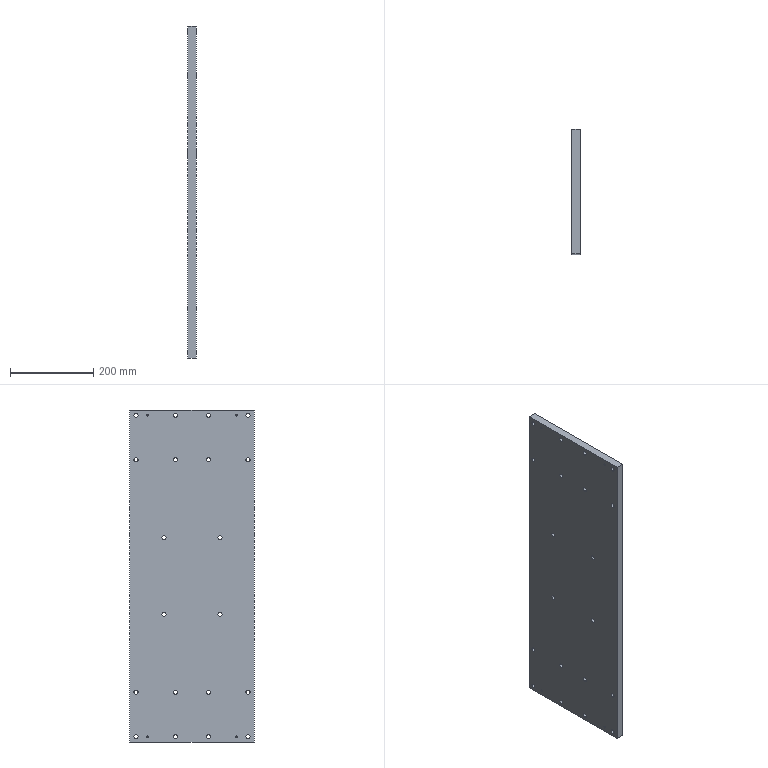Part | SolidWorks | features ICE 3, Extrusion 1 | 1 solid | 54 faces | box 20 x 300 x 800 mm | volume 4767476 mm3 | cylinder 48 | plane 6 | commonest cylinder face diameters 10 x40 4.2 x8